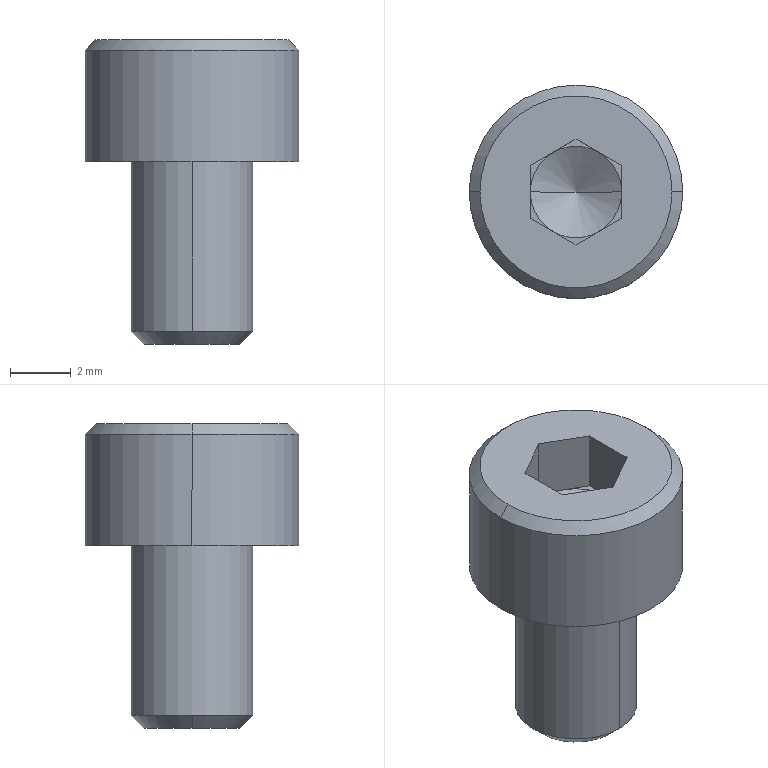Part | STEP file | 1 solid | 25 faces | box 7 x 7 x 10 mm | volume 209.329 mm3 | plane 15 | cone 6 | cylinder 4 | commonest cylinder face diameters 4 x2 7 x2